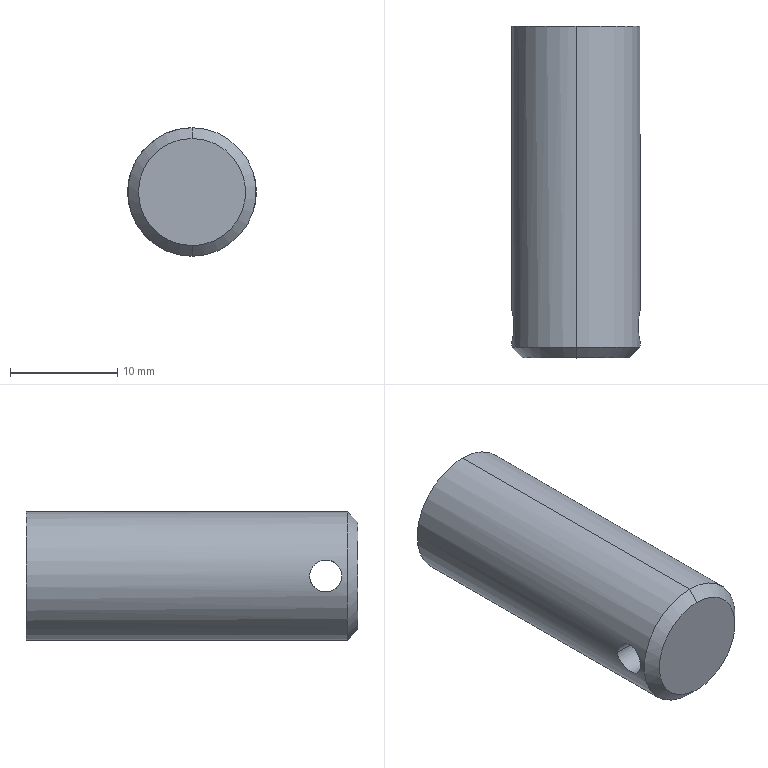Part | STEP file | Positioning_id990_x_t | 1 solid | 8 faces | box 12 x 31 x 12 mm | volume 3404 mm3 | cylinder 4 | cone 2 | plane 2 | commonest cylinder face diameters 3 x2 12 x2
STEP:
#1=CARTESIAN_POINT('',(0.,0.,0.));
#2=DIRECTION('',(0.,0.,1.));
#3=DIRECTION('',(1.,0.,0.));
#4=AXIS2_PLACEMENT_3D('',#1,#2,#3);
#5=CARTESIAN_POINT('',(-767.002,184.,187.532));
#6=VERTEX_POINT('',#5);
#7=CARTESIAN_POINT('',(-767.002,183.,188.532));
#8=VERTEX_POINT('',#7);
#9=CARTESIAN_POINT('',(-767.002,183.,188.532));
#10=DIRECTION('',(0.,-0.7071,0.7071));
#11=VECTOR('',#10,1.);
#12=LINE('',#9,#11);
#13=CARTESIAN_POINT('',(-767.002,184.,193.532));
#14=DIRECTION('',(0.,1.,0.));
#15=DIRECTION('',(0.,0.,-1.));
#16=AXIS2_PLACEMENT_3D('',#13,#14,#15);
#17=CONICAL_SURFACE('',#16,6.,0.7854);
#18=CARTESIAN_POINT('',(0.,-1.));
#19=DIRECTION('',(0.,-1.));
#20=VECTOR('',#19,1.);
#21=LINE('',#18,#20);
#22=(GEOMETRIC_REPRESENTATION_CONTEXT(2)PARAMETRIC_REPRESENTATION_CONTEXT()REPRESENTATION_CONTEXT('',''));
#23=DEFINITIONAL_REPRESENTATION('',(#21),#22);
#24=PCURVE('',#17,#23);
#25=CARTESIAN_POINT('',(-767.002,184.,193.532));
#26=DIRECTION('',(0.,1.,0.));
#27=DIRECTION('',(0.,0.,-1.));
#28=AXIS2_PLACEMENT_3D('',#25,#26,#27);
#29=CONICAL_SURFACE('',#28,6.,0.7854);
#30=CARTESIAN_POINT('',(6.283,-1.));
#31=DIRECTION('',(0.,-1.));
#32=VECTOR('',#31,1.);
#33=LINE('',#30,#32);
#34=(GEOMETRIC_REPRESENTATION_CONTEXT(2)PARAMETRIC_REPRESENTATION_CONTEXT()REPRESENTATION_CONTEXT('',''));
#35=DEFINITIONAL_REPRESENTATION('',(#33),#34);
#36=PCURVE('',#29,#35);
#37=SURFACE_CURVE('',#12,(#24,#36),.PCURVE_S1.);
#38=EDGE_CURVE('',#6,#8,#37,.T.);
#39=ORIENTED_EDGE('',*,*,#38,.T.);
#40=CARTESIAN_POINT('',(-767.002,183.,198.532));
#41=VERTEX_POINT('',#40);
#42=CARTESIAN_POINT('',(-767.002,183.,193.532));
#43=DIRECTION('',(0.,1.,0.));
#44=DIRECTION('',(0.,0.,1.));
#45=AXIS2_PLACEMENT_3D('',#42,#43,#44);
#46=CIRCLE('',#45,5.);
#47=CARTESIAN_POINT('',(-3.142,-1.));
#48=DIRECTION('',(1.,0.));
#49=VECTOR('',#48,1.);
#50=LINE('',#47,#49);
#51=(GEOMETRIC_REPRESENTATION_CONTEXT(2)PARAMETRIC_REPRESENTATION_CONTEXT()REPRESENTATION_CONTEXT('',''));
#52=DEFINITIONAL_REPRESENTATION('',(#50),#51);
#53=PCURVE('',#17,#52);
#54=CARTESIAN_POINT('',(-767.002,183.,193.532));
#55=DIRECTION('',(0.,-1.,0.));
#56=DIRECTION('',(0.,0.,-1.));
#57=AXIS2_PLACEMENT_3D('',#54,#55,#56);
#58=PLANE('',#57);
#59=CARTESIAN_POINT('',(-5.,0.));
#60=CARTESIAN_POINT('',(-5.,8.66));
#61=CARTESIAN_POINT('',(2.5,4.33));
#62=CARTESIAN_POINT('',(10.,0.));
#63=CARTESIAN_POINT('',(2.5,-4.33));
#64=CARTESIAN_POINT('',(-5.,-8.66));
#65=CARTESIAN_POINT('',(-5.,0.));
#66=(BOUNDED_CURVE()B_SPLINE_CURVE(2,(#59,#60,#61,#62,#63,#64,#65),.UNSPECIFIED.,.T.,.F.)B_SPLINE_CURVE_WITH_KNOTS((1,2,2,2,2,1),(-2.094,0.,2.094,4.189,6.283,8.378),.UNSPECIFIED.)CURVE()GEOMETRIC_REPRESENTATION_ITEM()RATIONAL_B_SPLINE_CURVE((1.,0.5,1.,0.5,1.,0.5,1.))REPRESENTATION_ITEM(''));
#67=(GEOMETRIC_REPRESENTATION_CONTEXT(2)PARAMETRIC_REPRESENTATION_CONTEXT()REPRESENTATION_CONTEXT('',''));
#68=DEFINITIONAL_REPRESENTATION('',(#66),#67);
#69=PCURVE('',#58,#68);
#70=SURFACE_CURVE('',#46,(#53,#69),.PCURVE_S1.);
#71=EDGE_CURVE('',#8,#41,#70,.T.);
#72=ORIENTED_EDGE('',*,*,#71,.T.);
#73=CARTESIAN_POINT('',(-767.002,184.,199.532));
#74=VERTEX_POINT('',#73);
#75=CARTESIAN_POINT('',(-767.002,183.,198.532));
#76=DIRECTION('',(0.,0.7071,0.7071));
#77=VECTOR('',#76,1.);
#78=LINE('',#75,#77);
#79=CARTESIAN_POINT('',(3.142,-1.));
#80=DIRECTION('',(0.,1.));
#81=VECTOR('',#80,1.);
#82=LINE('',#79,#81);
#83=(GEOMETRIC_REPRESENTATION_CONTEXT(2)PARAMETRIC_REPRESENTATION_CONTEXT()REPRESENTATION_CONTEXT('',''));
#84=DEFINITIONAL_REPRESENTATION('',(#82),#83);
#85=PCURVE('',#17,#84);
#86=CARTESIAN_POINT('',(3.142,-1.));
#87=DIRECTION('',(0.,1.));
#88=VECTOR('',#87,1.);
#89=LINE('',#86,#88);
#90=(GEOMETRIC_REPRESENTATION_CONTEXT(2)PARAMETRIC_REPRESENTATION_CONTEXT()REPRESENTATION_CONTEXT('',''));
#91=DEFINITIONAL_REPRESENTATION('',(#89),#90);
#92=PCURVE('',#29,#91);
#93=SURFACE_CURVE('',#78,(#85,#92),.PCURVE_S1.);
#94=EDGE_CURVE('',#41,#74,#93,.T.);
#95=ORIENTED_EDGE('',*,*,#94,.T.);
#96=CARTESIAN_POINT('',(-767.002,184.,193.532));
#97=DIRECTION('',(0.,-1.,0.));
#98=DIRECTION('',(0.,0.,1.));
#99=AXIS2_PLACEMENT_3D('',#96,#97,#98);
#100=CIRCLE('',#99,6.);
#101=CARTESIAN_POINT('',(3.142,0.));
#102=DIRECTION('',(-1.,0.));
#103=VECTOR('',#102,1.);
#104=LINE('',#101,#103);
#105=(GEOMETRIC_REPRESENTATION_CONTEXT(2)PARAMETRIC_REPRESENTATION_CONTEXT()REPRESENTATION_CONTEXT('',''));
#106=DEFINITIONAL_REPRESENTATION('',(#104),#105);
#107=PCURVE('',#17,#106);
#108=CARTESIAN_POINT('',(-767.002,214.,193.532));
#109=DIRECTION('',(0.,1.,0.));
#110=DIRECTION('',(0.,0.,-1.));
#111=AXIS2_PLACEMENT_3D('',#108,#109,#110);
#112=CYLINDRICAL_SURFACE('',#111,6.);
#113=CARTESIAN_POINT('',(3.142,-30.));
#114=DIRECTION('',(-1.,0.));
#115=VECTOR('',#114,1.);
#116=LINE('',#113,#115);
#117=(GEOMETRIC_REPRESENTATION_CONTEXT(2)PARAMETRIC_REPRESENTATION_CONTEXT()REPRESENTATION_CONTEXT('',''));
#118=DEFINITIONAL_REPRESENTATION('',(#116),#117);
#119=PCURVE('',#112,#118);
#120=SURFACE_CURVE('',#100,(#107,#119),.PCURVE_S1.);
#121=EDGE_CURVE('',#74,#6,#120,.T.);
#122=ORIENTED_EDGE('',*,*,#121,.T.);
#123=EDGE_LOOP('',(#39,#72,#95,#122));
#124=FACE_BOUND('',#123,.T.);
#125=ADVANCED_FACE('',(#124),#17,.T.);
#126=CARTESIAN_POINT('',(-773.002,184.5,193.532));
#127=VERTEX_POINT('',#126);
#128=CARTESIAN_POINT('',(-773.002,187.5,193.532));
#129=VERTEX_POINT('',#128);
#130=CARTESIAN_POINT('',(-773.002,184.5,193.532));
#131=CARTESIAN_POINT('',(-773.002,184.5,193.367));
#132=CARTESIAN_POINT('',(-772.995,184.528,193.2));
#133=CARTESIAN_POINT('',(-772.982,184.582,193.044));
#134=CARTESIAN_POINT('',(-772.969,184.635,192.888));
#135=CARTESIAN_POINT('',(-772.951,184.715,192.74));
#136=CARTESIAN_POINT('',(-772.931,184.816,192.611));
#137=CARTESIAN_POINT('',(-772.91,184.918,192.48));
#138=CARTESIAN_POINT('',(-772.888,185.044,192.364));
#139=CARTESIAN_POINT('',(-772.868,185.184,192.273));
#140=CARTESIAN_POINT('',(-772.849,185.326,192.181));
#141=CARTESIAN_POINT('',(-772.832,185.487,192.112));
#142=CARTESIAN_POINT('',(-772.822,185.652,192.073));
#143=CARTESIAN_POINT('',(-772.812,185.814,192.034));
#144=CARTESIAN_POINT('',(-772.809,185.986,192.023));
#145=CARTESIAN_POINT('',(-772.813,186.152,192.04));
#146=CARTESIAN_POINT('',(-772.818,186.314,192.056));
#147=CARTESIAN_POINT('',(-772.829,186.475,192.1));
#148=CARTESIAN_POINT('',(-772.845,186.623,192.167));
#149=CARTESIAN_POINT('',(-772.86,186.772,192.235));
#150=CARTESIAN_POINT('',(-772.881,186.911,192.329));
#151=CARTESIAN_POINT('',(-772.902,187.03,192.441));
#152=CARTESIAN_POINT('',(-772.923,187.152,192.557));
#153=CARTESIAN_POINT('',(-772.945,187.256,192.695));
#154=CARTESIAN_POINT('',(-772.962,187.333,192.844));
#155=CARTESIAN_POINT('',(-772.98,187.411,192.994));
#156=CARTESIAN_POINT('',(-772.993,187.463,193.161));
#157=CARTESIAN_POINT('',(-772.998,187.486,193.329));
#158=CARTESIAN_POINT('',(-773.001,187.495,193.396));
#159=CARTESIAN_POINT('',(-773.002,187.5,193.464));
#160=CARTESIAN_POINT('',(-773.002,187.5,193.532));
#161=B_SPLINE_CURVE_WITH_KNOTS('',3,(#130,#131,#132,#133,#134,#135,#136,#137,#138,#139,#140,#141,#142,#143,#144,#145,#146,#147,#148,#149,#150,#151,#152,#153,#154,#155,#156,#157,#158,#159,#160),.UNSPECIFIED.,.F.,.F.,(4,3,3,3,3,3,3,3,3,3,4),(0.,0.1052,0.2102,0.3173,0.4259,0.5324,0.6362,0.7411,0.849,0.9573,1.),.UNSPECIFIED.);
#162=CARTESIAN_POINT('',(-757.002,186.,193.532));
#163=DIRECTION('',(1.,0.,0.));
#164=DIRECTION('',(0.,-1.,0.));
#165=AXIS2_PLACEMENT_3D('',#162,#163,#164);
#166=CYLINDRICAL_SURFACE('',#165,1.5);
#167=CARTESIAN_POINT('',(0.,-16.));
#168=CARTESIAN_POINT('',(0.02377,-16.));
#169=CARTESIAN_POINT('',(0.07146,-15.999));
#170=CARTESIAN_POINT('',(0.1432,-15.996));
#171=CARTESIAN_POINT('',(0.215,-15.992));
#172=CARTESIAN_POINT('',(0.2866,-15.985));
#173=CARTESIAN_POINT('',(0.3577,-15.977));
#174=CARTESIAN_POINT('',(0.4291,-15.968));
#175=CARTESIAN_POINT('',(0.5006,-15.957));
#176=CARTESIAN_POINT('',(0.572,-15.945));
#177=CARTESIAN_POINT('',(0.6432,-15.932));
#178=CARTESIAN_POINT('',(0.714,-15.919));
#179=CARTESIAN_POINT('',(0.7852,-15.906));
#180=CARTESIAN_POINT('',(0.8564,-15.892));
#181=CARTESIAN_POINT('',(0.9277,-15.879));
#182=CARTESIAN_POINT('',(0.9986,-15.866));
#183=CARTESIAN_POINT('',(1.07,-15.854));
#184=CARTESIAN_POINT('',(1.141,-15.843));
#185=CARTESIAN_POINT('',(1.213,-15.833));
#186=CARTESIAN_POINT('',(1.284,-15.825));
#187=CARTESIAN_POINT('',(1.355,-15.818));
#188=CARTESIAN_POINT('',(1.427,-15.813));
#189=CARTESIAN_POINT('',(1.499,-15.81));
#190=CARTESIAN_POINT('',(1.57,-15.809));
#191=CARTESIAN_POINT('',(1.642,-15.81));
#192=CARTESIAN_POINT('',(1.713,-15.813));
#193=CARTESIAN_POINT('',(1.785,-15.818));
#194=CARTESIAN_POINT('',(1.857,-15.825));
#195=CARTESIAN_POINT('',(1.928,-15.833));
#196=CARTESIAN_POINT('',(1.999,-15.843));
#197=CARTESIAN_POINT('',(2.071,-15.854));
#198=CARTESIAN_POINT('',(2.142,-15.866));
#199=CARTESIAN_POINT('',(2.213,-15.879));
#200=CARTESIAN_POINT('',(2.285,-15.892));
#201=CARTESIAN_POINT('',(2.355,-15.905));
#202=CARTESIAN_POINT('',(2.426,-15.919));
#203=CARTESIAN_POINT('',(2.498,-15.932));
#204=CARTESIAN_POINT('',(2.569,-15.945));
#205=CARTESIAN_POINT('',(2.64,-15.957));
#206=CARTESIAN_POINT('',(2.711,-15.967));
#207=CARTESIAN_POINT('',(2.783,-15.977));
#208=CARTESIAN_POINT('',(2.854,-15.985));
#209=CARTESIAN_POINT('',(2.926,-15.992));
#210=CARTESIAN_POINT('',(2.997,-15.996));
#211=CARTESIAN_POINT('',(3.069,-15.999));
#212=CARTESIAN_POINT('',(3.118,-16.));
#213=CARTESIAN_POINT('',(3.142,-16.));
#214=B_SPLINE_CURVE_WITH_KNOTS('',3,(#167,#168,#169,#170,#171,#172,#173,#174,#175,#176,#177,#178,#179,#180,#181,#182,#183,#184,#185,#186,#187,#188,#189,#190,#191,#192,#193,#194,#195,#196,#197,#198,#199,#200,#201,#202,#203,#204,#205,#206,#207,#208,#209,#210,#211,#212,#213),.UNSPECIFIED.,.F.,.F.,(4,1,1,1,1,1,1,1,1,1,1,1,1,1,1,1,1,1,1,1,1,1,1,1,1,1,1,1,1,1,1,1,1,1,1,1,1,1,1,1,1,1,1,1,4),(0.,0.02273,0.04545,0.06818,0.09091,0.1136,0.1364,0.1591,0.1818,0.2045,0.2273,0.25,0.2727,0.2955,0.3182,0.3409,0.3636,0.3864,0.4091,0.4318,0.4545,0.4773,0.5,0.5227,0.5455,0.5682,0.5909,0.6136,0.6364,0.6591,0.6818,0.7045,0.7273,0.75,0.7727,0.7955,0.8182,0.8409,0.8636,0.8864,0.9091,0.9318,0.9545,0.9773,1.),.QUASI_UNIFORM_KNOTS.);
#215=(GEOMETRIC_REPRESENTATION_CONTEXT(2)PARAMETRIC_REPRESENTATION_CONTEXT()REPRESENTATION_CONTEXT('',''));
#216=DEFINITIONAL_REPRESENTATION('',(#214),#215);
#217=PCURVE('',#166,#216);
#218=CARTESIAN_POINT('',(1.571,-29.5));
#219=CARTESIAN_POINT('',(1.565,-29.5));
#220=CARTESIAN_POINT('',(1.553,-29.497));
#221=CARTESIAN_POINT('',(1.535,-29.486));
#222=CARTESIAN_POINT('',(1.517,-29.467));
#223=CARTESIAN_POINT('',(1.5,-29.44));
#224=CARTESIAN_POINT('',(1.483,-29.406));
#225=CARTESIAN_POINT('',(1.467,-29.365));
#226=CARTESIAN_POINT('',(1.45,-29.317));
#227=CARTESIAN_POINT('',(1.435,-29.262));
#228=CARTESIAN_POINT('',(1.42,-29.201));
#229=CARTESIAN_POINT('',(1.406,-29.135));
#230=CARTESIAN_POINT('',(1.393,-29.062));
#231=CARTESIAN_POINT('',(1.381,-28.983));
#232=CARTESIAN_POINT('',(1.369,-28.9));
#233=CARTESIAN_POINT('',(1.359,-28.813));
#234=CARTESIAN_POINT('',(1.35,-28.721));
#235=CARTESIAN_POINT('',(1.341,-28.625));
#236=CARTESIAN_POINT('',(1.334,-28.526));
#237=CARTESIAN_POINT('',(1.328,-28.425));
#238=CARTESIAN_POINT('',(1.324,-28.321));
#239=CARTESIAN_POINT('',(1.321,-28.216));
#240=CARTESIAN_POINT('',(1.319,-28.108));
#241=CARTESIAN_POINT('',(1.318,-28.001));
#242=CARTESIAN_POINT('',(1.319,-27.893));
#243=CARTESIAN_POINT('',(1.321,-27.787));
#244=CARTESIAN_POINT('',(1.324,-27.681));
#245=CARTESIAN_POINT('',(1.328,-27.577));
#246=CARTESIAN_POINT('',(1.334,-27.475));
#247=CARTESIAN_POINT('',(1.341,-27.376));
#248=CARTESIAN_POINT('',(1.349,-27.281));
#249=CARTESIAN_POINT('',(1.359,-27.188));
#250=CARTESIAN_POINT('',(1.369,-27.1));
#251=CARTESIAN_POINT('',(1.381,-27.017));
#252=CARTESIAN_POINT('',(1.393,-26.939));
#253=CARTESIAN_POINT('',(1.406,-26.867));
#254=CARTESIAN_POINT('',(1.42,-26.799));
#255=CARTESIAN_POINT('',(1.435,-26.738));
#256=CARTESIAN_POINT('',(1.45,-26.683));
#257=CARTESIAN_POINT('',(1.466,-26.636));
#258=CARTESIAN_POINT('',(1.483,-26.595));
#259=CARTESIAN_POINT('',(1.5,-26.56));
#260=CARTESIAN_POINT('',(1.517,-26.534));
#261=CARTESIAN_POINT('',(1.535,-26.514));
#262=CARTESIAN_POINT('',(1.553,-26.503));
#263=CARTESIAN_POINT('',(1.565,-26.5));
#264=CARTESIAN_POINT('',(1.571,-26.5));
#265=B_SPLINE_CURVE_WITH_KNOTS('',3,(#218,#219,#220,#221,#222,#223,#224,#225,#226,#227,#228,#229,#230,#231,#232,#233,#234,#235,#236,#237,#238,#239,#240,#241,#242,#243,#244,#245,#246,#247,#248,#249,#250,#251,#252,#253,#254,#255,#256,#257,#258,#259,#260,#261,#262,#263,#264),.UNSPECIFIED.,.F.,.F.,(4,1,1,1,1,1,1,1,1,1,1,1,1,1,1,1,1,1,1,1,1,1,1,1,1,1,1,1,1,1,1,1,1,1,1,1,1,1,1,1,1,1,1,1,4),(0.,0.02273,0.04545,0.06818,0.09091,0.1136,0.1364,0.1591,0.1818,0.2045,0.2273,0.25,0.2727,0.2955,0.3182,0.3409,0.3636,0.3864,0.4091,0.4318,0.4545,0.4773,0.5,0.5227,0.5455,0.5682,0.5909,0.6136,0.6364,0.6591,0.6818,0.7045,0.7273,0.75,0.7727,0.7955,0.8182,0.8409,0.8636,0.8864,0.9091,0.9318,0.9545,0.9773,1.),.QUASI_UNIFORM_KNOTS.);
#266=(GEOMETRIC_REPRESENTATION_CONTEXT(2)PARAMETRIC_REPRESENTATION_CONTEXT()REPRESENTATION_CONTEXT('',''));
#267=DEFINITIONAL_REPRESENTATION('',(#265),#266);
#268=PCURVE('',#112,#267);
#269=SURFACE_CURVE('',#161,(#217,#268),.PCURVE_S1.);
#270=EDGE_CURVE('',#127,#129,#269,.T.);
#271=ORIENTED_EDGE('',*,*,#270,.T.);
#272=CARTESIAN_POINT('',(-761.002,187.5,193.532));
#273=VERTEX_POINT('',#272);
#274=CARTESIAN_POINT('',(-761.002,187.5,193.532));
#275=DIRECTION('',(1.,0.,0.));
#276=VECTOR('',#275,1.);
#277=LINE('',#274,#276);
#278=CARTESIAN_POINT('',(3.142,-4.));
#279=DIRECTION('',(0.,1.));
#280=VECTOR('',#279,1.);
#281=LINE('',#278,#280);
#282=(GEOMETRIC_REPRESENTATION_CONTEXT(2)PARAMETRIC_REPRESENTATION_CONTEXT()REPRESENTATION_CONTEXT('',''));
#283=DEFINITIONAL_REPRESENTATION('',(#281),#282);
#284=PCURVE('',#166,#283);
#285=CARTESIAN_POINT('',(-757.002,186.,193.532));
#286=DIRECTION('',(1.,0.,0.));
#287=DIRECTION('',(0.,-1.,0.));
#288=AXIS2_PLACEMENT_3D('',#285,#286,#287);
#289=CYLINDRICAL_SURFACE('',#288,1.5);
#290=CARTESIAN_POINT('',(3.142,-4.));
#291=DIRECTION('',(0.,1.));
#292=VECTOR('',#291,1.);
#293=LINE('',#290,#292);
#294=(GEOMETRIC_REPRESENTATION_CONTEXT(2)PARAMETRIC_REPRESENTATION_CONTEXT()REPRESENTATION_CONTEXT('',''));
#295=DEFINITIONAL_REPRESENTATION('',(#293),#294);
#296=PCURVE('',#289,#295);
#297=SURFACE_CURVE('',#277,(#284,#296),.PCURVE_S1.);
#298=EDGE_CURVE('',#129,#273,#297,.T.);
#299=ORIENTED_EDGE('',*,*,#298,.T.);
#300=CARTESIAN_POINT('',(-761.002,184.5,193.532));
#301=VERTEX_POINT('',#300);
#302=CARTESIAN_POINT('',(-761.002,187.5,193.532));
#303=CARTESIAN_POINT('',(-761.002,187.5,193.367));
#304=CARTESIAN_POINT('',(-761.009,187.472,193.2));
#305=CARTESIAN_POINT('',(-761.022,187.418,193.044));
#306=CARTESIAN_POINT('',(-761.034,187.365,192.888));
#307=CARTESIAN_POINT('',(-761.053,187.285,192.74));
#308=CARTESIAN_POINT('',(-761.073,187.184,192.611));
#309=CARTESIAN_POINT('',(-761.093,187.082,192.48));
#310=CARTESIAN_POINT('',(-761.116,186.956,192.364));
#311=CARTESIAN_POINT('',(-761.135,186.816,192.273));
#312=CARTESIAN_POINT('',(-761.155,186.674,192.181));
#313=CARTESIAN_POINT('',(-761.172,186.513,192.112));
#314=CARTESIAN_POINT('',(-761.182,186.348,192.073));
#315=CARTESIAN_POINT('',(-761.192,186.186,192.034));
#316=CARTESIAN_POINT('',(-761.195,186.014,192.023));
#317=CARTESIAN_POINT('',(-761.19,185.848,192.04));
#318=CARTESIAN_POINT('',(-761.186,185.686,192.056));
#319=CARTESIAN_POINT('',(-761.175,185.525,192.1));
#320=CARTESIAN_POINT('',(-761.159,185.377,192.167));
#321=CARTESIAN_POINT('',(-761.143,185.228,192.235));
#322=CARTESIAN_POINT('',(-761.122,185.089,192.329));
#323=CARTESIAN_POINT('',(-761.102,184.97,192.441));
#324=CARTESIAN_POINT('',(-761.08,184.848,192.557));
#325=CARTESIAN_POINT('',(-761.059,184.744,192.695));
#326=CARTESIAN_POINT('',(-761.041,184.667,192.844));
#327=CARTESIAN_POINT('',(-761.024,184.589,192.994));
#328=CARTESIAN_POINT('',(-761.011,184.537,193.161));
#329=CARTESIAN_POINT('',(-761.005,184.514,193.329));
#330=CARTESIAN_POINT('',(-761.003,184.505,193.396));
#331=CARTESIAN_POINT('',(-761.002,184.5,193.464));
#332=CARTESIAN_POINT('',(-761.002,184.5,193.532));
#333=B_SPLINE_CURVE_WITH_KNOTS('',3,(#302,#303,#304,#305,#306,#307,#308,#309,#310,#311,#312,#313,#314,#315,#316,#317,#318,#319,#320,#321,#322,#323,#324,#325,#326,#327,#328,#329,#330,#331,#332),.UNSPECIFIED.,.F.,.F.,(4,3,3,3,3,3,3,3,3,3,4),(0.,0.1052,0.2102,0.3173,0.4259,0.5324,0.6362,0.7411,0.849,0.9573,1.),.UNSPECIFIED.);
#334=CARTESIAN_POINT('',(3.142,-4.));
#335=CARTESIAN_POINT('',(3.118,-4.));
#336=CARTESIAN_POINT('',(3.07,-4.001));
#337=CARTESIAN_POINT('',(2.998,-4.004));
#338=CARTESIAN_POINT('',(2.927,-4.008));
#339=CARTESIAN_POINT('',(2.855,-4.015));
#340=CARTESIAN_POINT('',(2.784,-4.023));
#341=CARTESIAN_POINT('',(2.712,-4.032));
#342=CARTESIAN_POINT('',(2.641,-4.043));
#343=CARTESIAN_POINT('',(2.57,-4.055));
#344=CARTESIAN_POINT('',(2.498,-4.068));
#345=CARTESIAN_POINT('',(2.428,-4.081));
#346=CARTESIAN_POINT('',(2.356,-4.094));
#347=CARTESIAN_POINT('',(2.285,-4.108));
#348=CARTESIAN_POINT('',(2.214,-4.121));
#349=CARTESIAN_POINT('',(2.143,-4.134));
#350=CARTESIAN_POINT('',(2.072,-4.146));
#351=CARTESIAN_POINT('',(2.001,-4.157));
#352=CARTESIAN_POINT('',(1.929,-4.167));
#353=CARTESIAN_POINT('',(1.858,-4.175));
#354=CARTESIAN_POINT('',(1.786,-4.182));
#355=CARTESIAN_POINT('',(1.715,-4.187));
#356=CARTESIAN_POINT('',(1.643,-4.19));
#357=CARTESIAN_POINT('',(1.571,-4.191));
#358=CARTESIAN_POINT('',(1.5,-4.19));
#359=CARTESIAN_POINT('',(1.428,-4.187));
#360=CARTESIAN_POINT('',(1.357,-4.182));
#361=CARTESIAN_POINT('',(1.285,-4.175));
#362=CARTESIAN_POINT('',(1.213,-4.167));
#363=CARTESIAN_POINT('',(1.142,-4.157));
#364=CARTESIAN_POINT('',(1.071,-4.146));
#365=CARTESIAN_POINT('',(0.9996,-4.134));
#366=CARTESIAN_POINT('',(0.9282,-4.121));
#367=CARTESIAN_POINT('',(0.857,-4.108));
#368=CARTESIAN_POINT('',(0.7863,-4.095));
#369=CARTESIAN_POINT('',(0.7152,-4.081));
#370=CARTESIAN_POINT('',(0.6439,-4.068));
#371=CARTESIAN_POINT('',(0.5726,-4.055));
#372=CARTESIAN_POINT('',(0.5014,-4.043));
#373=CARTESIAN_POINT('',(0.4305,-4.033));
#374=CARTESIAN_POINT('',(0.359,-4.023));
#375=CARTESIAN_POINT('',(0.2874,-4.015));
#376=CARTESIAN_POINT('',(0.2157,-4.008));
#377=CARTESIAN_POINT('',(0.1445,-4.004));
#378=CARTESIAN_POINT('',(0.07225,-4.001));
#379=CARTESIAN_POINT('',(0.02405,-4.));
#380=CARTESIAN_POINT('',(0.,-4.));
#381=B_SPLINE_CURVE_WITH_KNOTS('',3,(#334,#335,#336,#337,#338,#339,#340,#341,#342,#343,#344,#345,#346,#347,#348,#349,#350,#351,#352,#353,#354,#355,#356,#357,#358,#359,#360,#361,#362,#363,#364,#365,#366,#367,#368,#369,#370,#371,#372,#373,#374,#375,#376,#377,#378,#379,#380),.UNSPECIFIED.,.F.,.F.,(4,1,1,1,1,1,1,1,1,1,1,1,1,1,1,1,1,1,1,1,1,1,1,1,1,1,1,1,1,1,1,1,1,1,1,1,1,1,1,1,1,1,1,1,4),(0.,0.02273,0.04545,0.06818,0.09091,0.1136,0.1364,0.1591,0.1818,0.2045,0.2273,0.25,0.2727,0.2955,0.3182,0.3409,0.3636,0.3864,0.4091,0.4318,0.4545,0.4773,0.5,0.5227,0.5455,0.5682,0.5909,0.6136,0.6364,0.6591,0.6818,0.7045,0.7273,0.75,0.7727,0.7955,0.8182,0.8409,0.8636,0.8864,0.9091,0.9318,0.9545,0.9773,1.),.QUASI_UNIFORM_KNOTS.);
#382=(GEOMETRIC_REPRESENTATION_CONTEXT(2)PARAMETRIC_REPRESENTATION_CONTEXT()REPRESENTATION_CONTEXT('',''));
#383=DEFINITIONAL_REPRESENTATION('',(#381),#382);
#384=PCURVE('',#166,#383);
#385=CARTESIAN_POINT('',(-767.002,214.,193.532));
#386=DIRECTION('',(0.,1.,0.));
#387=DIRECTION('',(0.,0.,-1.));
#388=AXIS2_PLACEMENT_3D('',#385,#386,#387);
#389=CYLINDRICAL_SURFACE('',#388,6.);
#390=CARTESIAN_POINT('',(4.712,-26.5));
#391=CARTESIAN_POINT('',(4.718,-26.5));
#392=CARTESIAN_POINT('',(4.73,-26.503));
#393=CARTESIAN_POINT('',(4.748,-26.514));
#394=CARTESIAN_POINT('',(4.766,-26.533));
#395=CARTESIAN_POINT('',(4.783,-26.56));
#396=CARTESIAN_POINT('',(4.8,-26.594));
#397=CARTESIAN_POINT('',(4.817,-26.635));
#398=CARTESIAN_POINT('',(4.833,-26.683));
#399=CARTESIAN_POINT('',(4.848,-26.738));
#400=CARTESIAN_POINT('',(4.863,-26.799));
#401=CARTESIAN_POINT('',(4.877,-26.865));
#402=CARTESIAN_POINT('',(4.89,-26.938));
#403=CARTESIAN_POINT('',(4.903,-27.017));
#404=CARTESIAN_POINT('',(4.914,-27.1));
#405=CARTESIAN_POINT('',(4.924,-27.187));
#406=CARTESIAN_POINT('',(4.934,-27.279));
#407=CARTESIAN_POINT('',(4.942,-27.375));
#408=CARTESIAN_POINT('',(4.949,-27.474));
#409=CARTESIAN_POINT('',(4.955,-27.575));
#410=CARTESIAN_POINT('',(4.959,-27.679));
#411=CARTESIAN_POINT('',(4.963,-27.784));
#412=CARTESIAN_POINT('',(4.965,-27.892));
#413=CARTESIAN_POINT('',(4.965,-27.999));
#414=CARTESIAN_POINT('',(4.965,-28.107));
#415=CARTESIAN_POINT('',(4.963,-28.213));
#416=CARTESIAN_POINT('',(4.959,-28.319));
#417=CARTESIAN_POINT('',(4.955,-28.423));
#418=CARTESIAN_POINT('',(4.949,-28.525));
#419=CARTESIAN_POINT('',(4.942,-28.624));
#420=CARTESIAN_POINT('',(4.934,-28.719));
#421=CARTESIAN_POINT('',(4.924,-28.812));
#422=CARTESIAN_POINT('',(4.914,-28.9));
#423=CARTESIAN_POINT('',(4.903,-28.983));
#424=CARTESIAN_POINT('',(4.89,-29.061));
#425=CARTESIAN_POINT('',(4.877,-29.133));
#426=CARTESIAN_POINT('',(4.863,-29.201));
#427=CARTESIAN_POINT('',(4.848,-29.262));
#428=CARTESIAN_POINT('',(4.833,-29.317));
#429=CARTESIAN_POINT('',(4.817,-29.364));
#430=CARTESIAN_POINT('',(4.8,-29.405));
#431=CARTESIAN_POINT('',(4.783,-29.44));
#432=CARTESIAN_POINT('',(4.766,-29.466));
#433=CARTESIAN_POINT('',(4.748,-29.486));
#434=CARTESIAN_POINT('',(4.73,-29.497));
#435=CARTESIAN_POINT('',(4.718,-29.5));
#436=CARTESIAN_POINT('',(4.712,-29.5));
#437=B_SPLINE_CURVE_WITH_KNOTS('',3,(#390,#391,#392,#393,#394,#395,#396,#397,#398,#399,#400,#401,#402,#403,#404,#405,#406,#407,#408,#409,#410,#411,#412,#413,#414,#415,#416,#417,#418,#419,#420,#421,#422,#423,#424,#425,#426,#427,#428,#429,#430,#431,#432,#433,#434,#435,#436),.UNSPECIFIED.,.F.,.F.,(4,1,1,1,1,1,1,1,1,1,1,1,1,1,1,1,1,1,1,1,1,1,1,1,1,1,1,1,1,1,1,1,1,1,1,1,1,1,1,1,1,1,1,1,4),(0.,0.02273,0.04545,0.06818,0.09091,0.1136,0.1364,0.1591,0.1818,0.2045,0.2273,0.25,0.2727,0.2955,0.3182,0.3409,0.3636,0.3864,0.4091,0.4318,0.4545,0.4773,0.5,0.5227,0.5455,0.5682,0.5909,0.6136,0.6364,0.6591,0.6818,0.7045,0.7273,0.75,0.7727,0.7955,0.8182,0.8409,0.8636,0.8864,0.9091,0.9318,0.9545,0.9773,1.),.QUASI_UNIFORM_KNOTS.);
#438=(GEOMETRIC_REPRESENTATION_CONTEXT(2)PARAMETRIC_REPRESENTATION_CONTEXT()REPRESENTATION_CONTEXT('',''));
#439=DEFINITIONAL_REPRESENTATION('',(#437),#438);
#440=PCURVE('',#389,#439);
#441=SURFACE_CURVE('',#333,(#384,#440),.PCURVE_S1.);
#442=EDGE_CURVE('',#273,#301,#441,.T.);
#443=ORIENTED_EDGE('',*,*,#442,.T.);
#444=CARTESIAN_POINT('',(-761.002,184.5,193.532));
#445=DIRECTION('',(-1.,0.,0.));
#446=VECTOR('',#445,1.);
#447=LINE('',#444,#446);
#448=CARTESIAN_POINT('',(0.,-4.));
#449=DIRECTION('',(0.,-1.));
#450=VECTOR('',#449,1.);
#451=LINE('',#448,#450);
#452=(GEOMETRIC_REPRESENTATION_CONTEXT(2)PARAMETRIC_REPRESENTATION_CONTEXT()REPRESENTATION_CONTEXT('',''));
#453=DEFINITIONAL_REPRESENTATION('',(#451),#452);
#454=PCURVE('',#166,#453);
#455=CARTESIAN_POINT('',(6.283,-4.));
#456=DIRECTION('',(0.,-1.));
#457=VECTOR('',#456,1.);
#458=LINE('',#455,#457);
#459=(GEOMETRIC_REPRESENTATION_CONTEXT(2)PARAMETRIC_REPRESENTATION_CONTEXT()REPRESENTATION_CONTEXT('',''));
#460=DEFINITIONAL_REPRESENTATION('',(#458),#459);
#461=PCURVE('',#289,#460);
#462=SURFACE_CURVE('',#447,(#454,#461),.PCURVE_S1.);
#463=EDGE_CURVE('',#301,#127,#462,.T.);
#464=ORIENTED_EDGE('',*,*,#463,.T.);
#465=EDGE_LOOP('',(#271,#299,#443,#464));
#466=FACE_BOUND('',#465,.F.);
#467=ADVANCED_FACE('',(#466),#166,.F.);
#468=ORIENTED_EDGE('',*,*,#442,.T.);
#469=CARTESIAN_POINT('',(-761.002,184.5,193.532));
#470=CARTESIAN_POINT('',(-761.002,184.5,193.697));
#471=CARTESIAN_POINT('',(-761.009,184.528,193.864));
#472=CARTESIAN_POINT('',(-761.022,184.582,194.02));
#473=CARTESIAN_POINT('',(-761.034,184.635,194.175));
#474=CARTESIAN_POINT('',(-761.053,184.715,194.323));
#475=CARTESIAN_POINT('',(-761.073,184.816,194.453));
#476=CARTESIAN_POINT('',(-761.093,184.918,194.584));
#477=CARTESIAN_POINT('',(-761.116,185.044,194.7));
#478=CARTESIAN_POINT('',(-761.135,185.184,194.791));
#479=CARTESIAN_POINT('',(-761.155,185.326,194.883));
#480=CARTESIAN_POINT('',(-761.172,185.487,194.952));
#481=CARTESIAN_POINT('',(-761.182,185.652,194.991));
#482=CARTESIAN_POINT('',(-761.192,185.814,195.03));
#483=CARTESIAN_POINT('',(-761.195,185.986,195.041));
#484=CARTESIAN_POINT('',(-761.19,186.152,195.024));
#485=CARTESIAN_POINT('',(-761.186,186.314,195.008));
#486=CARTESIAN_POINT('',(-761.175,186.475,194.964));
#487=CARTESIAN_POINT('',(-761.159,186.623,194.896));
#488=CARTESIAN_POINT('',(-761.143,186.772,194.828));
#489=CARTESIAN_POINT('',(-761.122,186.911,194.735));
#490=CARTESIAN_POINT('',(-761.102,187.03,194.623));
#491=CARTESIAN_POINT('',(-761.08,187.152,194.507));
#492=CARTESIAN_POINT('',(-761.059,187.256,194.369));
#493=CARTESIAN_POINT('',(-761.041,187.333,194.219));
#494=CARTESIAN_POINT('',(-761.024,187.411,194.069));
#495=CARTESIAN_POINT('',(-761.011,187.463,193.903));
#496=CARTESIAN_POINT('',(-761.005,187.486,193.735));
#497=CARTESIAN_POINT('',(-761.003,187.495,193.668));
#498=CARTESIAN_POINT('',(-761.002,187.5,193.6));
#499=CARTESIAN_POINT('',(-761.002,187.5,193.532));
#500=B_SPLINE_CURVE_WITH_KNOTS('',3,(#469,#470,#471,#472,#473,#474,#475,#476,#477,#478,#479,#480,#481,#482,#483,#484,#485,#486,#487,#488,#489,#490,#491,#492,#493,#494,#495,#496,#497,#498,#499),.UNSPECIFIED.,.F.,.F.,(4,3,3,3,3,3,3,3,3,3,4),(0.,0.1052,0.2102,0.3173,0.4259,0.5324,0.6362,0.7411,0.849,0.9573,1.),.UNSPECIFIED.);
#501=CARTESIAN_POINT('',(4.712,-29.5));
#502=CARTESIAN_POINT('',(4.706,-29.5));
#503=CARTESIAN_POINT('',(4.695,-29.497));
#504=CARTESIAN_POINT('',(4.677,-29.486));
#505=CARTESIAN_POINT('',(4.659,-29.467));
#506=CARTESIAN_POINT('',(4.642,-29.44));
#507=CARTESIAN_POINT('',(4.625,-29.406));
#508=CARTESIAN_POINT('',(4.608,-29.365));
#509=CARTESIAN_POINT('',(4.592,-29.317));
#510=CARTESIAN_POINT('',(4.577,-29.262));
#511=CARTESIAN_POINT('',(4.562,-29.201));
#512=CARTESIAN_POINT('',(4.548,-29.135));
#513=CARTESIAN_POINT('',(4.535,-29.062));
#514=CARTESIAN_POINT('',(4.522,-28.983));
#515=CARTESIAN_POINT('',(4.511,-28.9));
#516=CARTESIAN_POINT('',(4.5,-28.813));
#517=CARTESIAN_POINT('',(4.491,-28.721));
#518=CARTESIAN_POINT('',(4.483,-28.625));
#519=CARTESIAN_POINT('',(4.476,-28.526));
#520=CARTESIAN_POINT('',(4.47,-28.425));
#521=CARTESIAN_POINT('',(4.465,-28.321));
#522=CARTESIAN_POINT('',(4.462,-28.216));
#523=CARTESIAN_POINT('',(4.46,-28.108));
#524=CARTESIAN_POINT('',(4.46,-28.001));
#525=CARTESIAN_POINT('',(4.46,-27.893));
#526=CARTESIAN_POINT('',(4.462,-27.787));
#527=CARTESIAN_POINT('',(4.465,-27.681));
#528=CARTESIAN_POINT('',(4.47,-27.577));
#529=CARTESIAN_POINT('',(4.476,-27.475));
#530=CARTESIAN_POINT('',(4.483,-27.376));
#531=CARTESIAN_POINT('',(4.491,-27.281));
#532=CARTESIAN_POINT('',(4.5,-27.188));
#533=CARTESIAN_POINT('',(4.511,-27.1));
#534=CARTESIAN_POINT('',(4.522,-27.017));
#535=CARTESIAN_POINT('',(4.534,-26.939));
#536=CARTESIAN_POINT('',(4.548,-26.867));
#537=CARTESIAN_POINT('',(4.562,-26.799));
#538=CARTESIAN_POINT('',(4.576,-26.738));
#539=CARTESIAN_POINT('',(4.592,-26.683));
#540=CARTESIAN_POINT('',(4.608,-26.636));
#541=CARTESIAN_POINT('',(4.624,-26.595));
#542=CARTESIAN_POINT('',(4.641,-26.56));
#543=CARTESIAN_POINT('',(4.659,-26.534));
#544=CARTESIAN_POINT('',(4.676,-26.514));
#545=CARTESIAN_POINT('',(4.694,-26.503));
#546=CARTESIAN_POINT('',(4.706,-26.5));
#547=CARTESIAN_POINT('',(4.712,-26.5));
#548=B_SPLINE_CURVE_WITH_KNOTS('',3,(#501,#502,#503,#504,#505,#506,#507,#508,#509,#510,#511,#512,#513,#514,#515,#516,#517,#518,#519,#520,#521,#522,#523,#524,#525,#526,#527,#528,#529,#530,#531,#532,#533,#534,#535,#536,#537,#538,#539,#540,#541,#542,#543,#544,#545,#546,#547),.UNSPECIFIED.,.F.,.F.,(4,1,1,1,1,1,1,1,1,1,1,1,1,1,1,1,1,1,1,1,1,1,1,1,1,1,1,1,1,1,1,1,1,1,1,1,1,1,1,1,1,1,1,1,4),(0.,0.02273,0.04545,0.06818,0.09091,0.1136,0.1364,0.1591,0.1818,0.2045,0.2273,0.25,0.2727,0.2955,0.3182,0.3409,0.3636,0.3864,0.4091,0.4318,0.4545,0.4773,0.5,0.5227,0.5455,0.5682,0.5909,0.6136,0.6364,0.6591,0.6818,0.7045,0.7273,0.75,0.7727,0.7955,0.8182,0.8409,0.8636,0.8864,0.9091,0.9318,0.9545,0.9773,1.),.QUASI_UNIFORM_KNOTS.);
#549=(GEOMETRIC_REPRESENTATION_CONTEXT(2)PARAMETRIC_REPRESENTATION_CONTEXT()REPRESENTATION_CONTEXT('',''));
#550=DEFINITIONAL_REPRESENTATION('',(#548),#549);
#551=PCURVE('',#389,#550);
#552=CARTESIAN_POINT('',(6.283,-4.));
#553=CARTESIAN_POINT('',(6.259,-4.));
#554=CARTESIAN_POINT('',(6.212,-4.001));
#555=CARTESIAN_POINT('',(6.14,-4.004));
#556=CARTESIAN_POINT('',(6.068,-4.008));
#557=CARTESIAN_POINT('',(5.997,-4.015));
#558=CARTESIAN_POINT('',(5.925,-4.023));
#559=CARTESIAN_POINT('',(5.854,-4.032));
#560=CARTESIAN_POINT('',(5.783,-4.043));
#561=CARTESIAN_POINT('',(5.711,-4.055));
#562=CARTESIAN_POINT('',(5.64,-4.068));
#563=CARTESIAN_POINT('',(5.569,-4.081));
#564=CARTESIAN_POINT('',(5.498,-4.094));
#565=CARTESIAN_POINT('',(5.427,-4.108));
#566=CARTESIAN_POINT('',(5.355,-4.121));
#567=CARTESIAN_POINT('',(5.285,-4.134));
#568=CARTESIAN_POINT('',(5.214,-4.146));
#569=CARTESIAN_POINT('',(5.142,-4.157));
#570=CARTESIAN_POINT('',(5.071,-4.167));
#571=CARTESIAN_POINT('',(4.999,-4.175));
#572=CARTESIAN_POINT('',(4.928,-4.182));
#573=CARTESIAN_POINT('',(4.856,-4.187));
#574=CARTESIAN_POINT('',(4.785,-4.19));
#575=CARTESIAN_POINT('',(4.713,-4.191));
#576=CARTESIAN_POINT('',(4.641,-4.19));
#577=CARTESIAN_POINT('',(4.57,-4.187));
#578=CARTESIAN_POINT('',(4.498,-4.182));
#579=CARTESIAN_POINT('',(4.427,-4.175));
#580=CARTESIAN_POINT('',(4.355,-4.167));
#581=CARTESIAN_POINT('',(4.284,-4.157));
#582=CARTESIAN_POINT('',(4.213,-4.146));
#583=CARTESIAN_POINT('',(4.141,-4.134));
#584=CARTESIAN_POINT('',(4.07,-4.121));
#585=CARTESIAN_POINT('',(3.999,-4.108));
#586=CARTESIAN_POINT('',(3.928,-4.095));
#587=CARTESIAN_POINT('',(3.857,-4.081));
#588=CARTESIAN_POINT('',(3.785,-4.068));
#589=CARTESIAN_POINT('',(3.714,-4.055));
#590=CARTESIAN_POINT('',(3.643,-4.043));
#591=CARTESIAN_POINT('',(3.572,-4.033));
#592=CARTESIAN_POINT('',(3.501,-4.023));
#593=CARTESIAN_POINT('',(3.429,-4.015));
#594=CARTESIAN_POINT('',(3.357,-4.008));
#595=CARTESIAN_POINT('',(3.286,-4.004));
#596=CARTESIAN_POINT('',(3.214,-4.001));
#597=CARTESIAN_POINT('',(3.166,-4.));
#598=CARTESIAN_POINT('',(3.142,-4.));
#599=B_SPLINE_CURVE_WITH_KNOTS('',3,(#552,#553,#554,#555,#556,#557,#558,#559,#560,#561,#562,#563,#564,#565,#566,#567,#568,#569,#570,#571,#572,#573,#574,#575,#576,#577,#578,#579,#580,#581,#582,#583,#584,#585,#586,#587,#588,#589,#590,#591,#592,#593,#594,#595,#596,#597,#598),.UNSPECIFIED.,.F.,.F.,(4,1,1,1,1,1,1,1,1,1,1,1,1,1,1,1,1,1,1,1,1,1,1,1,1,1,1,1,1,1,1,1,1,1,1,1,1,1,1,1,1,1,1,1,4),(0.,0.02273,0.04545,0.06818,0.09091,0.1136,0.1364,0.1591,0.1818,0.2045,0.2273,0.25,0.2727,0.2955,0.3182,0.3409,0.3636,0.3864,0.4091,0.4318,0.4545,0.4773,0.5,0.5227,0.5455,0.5682,0.5909,0.6136,0.6364,0.6591,0.6818,0.7045,0.7273,0.75,0.7727,0.7955,0.8182,0.8409,0.8636,0.8864,0.9091,0.9318,0.9545,0.9773,1.),.QUASI_UNIFORM_KNOTS.);
#600=(GEOMETRIC_REPRESENTATION_CONTEXT(2)PARAMETRIC_REPRESENTATION_CONTEXT()REPRESENTATION_CONTEXT('',''));
#601=DEFINITIONAL_REPRESENTATION('',(#599),#600);
#602=PCURVE('',#289,#601);
#603=SURFACE_CURVE('',#500,(#551,#602),.PCURVE_S1.);
#604=EDGE_CURVE('',#301,#273,#603,.T.);
#605=ORIENTED_EDGE('',*,*,#604,.T.);
#606=EDGE_LOOP('',(#468,#605));
#607=FACE_BOUND('',#606,.T.);
#608=CARTESIAN_POINT('',(-767.002,214.,187.532));
#609=VERTEX_POINT('',#608);
#610=CARTESIAN_POINT('',(-767.002,214.,187.532));
#611=DIRECTION('',(0.,1.,0.));
#612=VECTOR('',#611,1.);
#613=LINE('',#610,#612);
#614=CARTESIAN_POINT('',(6.283,0.));
#615=DIRECTION('',(0.,1.));
#616=VECTOR('',#615,1.);
#617=LINE('',#614,#616);
#618=(GEOMETRIC_REPRESENTATION_CONTEXT(2)PARAMETRIC_REPRESENTATION_CONTEXT()REPRESENTATION_CONTEXT('',''));
#619=DEFINITIONAL_REPRESENTATION('',(#617),#618);
#620=PCURVE('',#389,#619);
#621=CARTESIAN_POINT('',(0.,0.));
#622=DIRECTION('',(0.,1.));
#623=VECTOR('',#622,1.);
#624=LINE('',#621,#623);
#625=(GEOMETRIC_REPRESENTATION_CONTEXT(2)PARAMETRIC_REPRESENTATION_CONTEXT()REPRESENTATION_CONTEXT('',''));
#626=DEFINITIONAL_REPRESENTATION('',(#624),#625);
#627=PCURVE('',#112,#626);
#628=SURFACE_CURVE('',#613,(#620,#627),.PCURVE_S1.);
#629=EDGE_CURVE('',#6,#609,#628,.T.);
#630=ORIENTED_EDGE('',*,*,#629,.T.);
#631=CARTESIAN_POINT('',(-767.002,214.,199.532));
#632=VERTEX_POINT('',#631);
#633=CARTESIAN_POINT('',(-767.002,214.,193.532));
#634=DIRECTION('',(0.,1.,0.));
#635=DIRECTION('',(0.,0.,1.));
#636=AXIS2_PLACEMENT_3D('',#633,#634,#635);
#637=CIRCLE('',#636,6.);
#638=CARTESIAN_POINT('',(3.142,0.));
#639=DIRECTION('',(1.,0.));
#640=VECTOR('',#639,1.);
#641=LINE('',#638,#640);
#642=(GEOMETRIC_REPRESENTATION_CONTEXT(2)PARAMETRIC_REPRESENTATION_CONTEXT()REPRESENTATION_CONTEXT('',''));
#643=DEFINITIONAL_REPRESENTATION('',(#641),#642);
#644=PCURVE('',#389,#643);
#645=CARTESIAN_POINT('',(-767.002,214.,193.532));
#646=DIRECTION('',(0.,1.,0.));
#647=DIRECTION('',(0.,0.,1.));
#648=AXIS2_PLACEMENT_3D('',#645,#646,#647);
#649=PLANE('',#648);
#650=CARTESIAN_POINT('',(0.,0.));
#651=DIRECTION('',(1.,0.));
#652=AXIS2_PLACEMENT_2D('',#650,#651);
#653=CIRCLE('',#652,6.);
#654=(GEOMETRIC_REPRESENTATION_CONTEXT(2)PARAMETRIC_REPRESENTATION_CONTEXT()REPRESENTATION_CONTEXT('',''));
#655=DEFINITIONAL_REPRESENTATION('',(#653),#654);
#656=PCURVE('',#649,#655);
#657=SURFACE_CURVE('',#637,(#644,#656),.PCURVE_S1.);
#658=EDGE_CURVE('',#632,#609,#657,.T.);
#659=ORIENTED_EDGE('',*,*,#658,.F.);
#660=CARTESIAN_POINT('',(-767.002,214.,199.532));
#661=DIRECTION('',(0.,-1.,0.));
#662=VECTOR('',#661,1.);
#663=LINE('',#660,#662);
#664=CARTESIAN_POINT('',(3.142,0.));
#665=DIRECTION('',(0.,-1.));
#666=VECTOR('',#665,1.);
#667=LINE('',#664,#666);
#668=(GEOMETRIC_REPRESENTATION_CONTEXT(2)PARAMETRIC_REPRESENTATION_CONTEXT()REPRESENTATION_CONTEXT('',''));
#669=DEFINITIONAL_REPRESENTATION('',(#667),#668);
#670=PCURVE('',#389,#669);
#671=CARTESIAN_POINT('',(3.142,0.));
#672=DIRECTION('',(0.,-1.));
#673=VECTOR('',#672,1.);
#674=LINE('',#671,#673);
#675=(GEOMETRIC_REPRESENTATION_CONTEXT(2)PARAMETRIC_REPRESENTATION_CONTEXT()REPRESENTATION_CONTEXT('',''));
#676=DEFINITIONAL_REPRESENTATION('',(#674),#675);
#677=PCURVE('',#112,#676);
#678=SURFACE_CURVE('',#663,(#670,#677),.PCURVE_S1.);
#679=EDGE_CURVE('',#632,#74,#678,.T.);
#680=ORIENTED_EDGE('',*,*,#679,.T.);
#681=CARTESIAN_POINT('',(-767.002,184.,193.532));
#682=DIRECTION('',(0.,-1.,0.));
#683=DIRECTION('',(0.,0.,-1.));
#684=AXIS2_PLACEMENT_3D('',#681,#682,#683);
#685=CIRCLE('',#684,6.);
#686=CARTESIAN_POINT('',(6.283,-30.));
#687=DIRECTION('',(-1.,0.));
#688=VECTOR('',#687,1.);
#689=LINE('',#686,#688);
#690=(GEOMETRIC_REPRESENTATION_CONTEXT(2)PARAMETRIC_REPRESENTATION_CONTEXT()REPRESENTATION_CONTEXT('',''));
#691=DEFINITIONAL_REPRESENTATION('',(#689),#690);
#692=PCURVE('',#389,#691);
#693=CARTESIAN_POINT('',(6.283,0.));
#694=DIRECTION('',(-1.,0.));
#695=VECTOR('',#694,1.);
#696=LINE('',#693,#695);
#697=(GEOMETRIC_REPRESENTATION_CONTEXT(2)PARAMETRIC_REPRESENTATION_CONTEXT()REPRESENTATION_CONTEXT('',''));
#698=DEFINITIONAL_REPRESENTATION('',(#696),#697);
#699=PCURVE('',#29,#698);
#700=SURFACE_CURVE('',#685,(#692,#699),.PCURVE_S1.);
#701=EDGE_CURVE('',#6,#74,#700,.T.);
#702=ORIENTED_EDGE('',*,*,#701,.F.);
#703=EDGE_LOOP('',(#630,#659,#680,#702));
#704=FACE_BOUND('',#703,.T.);
#705=ADVANCED_FACE('',(#607,#704),#389,.T.);
#706=ORIENTED_EDGE('',*,*,#658,.T.);
#707=CARTESIAN_POINT('',(-767.002,214.,187.532));
#708=CARTESIAN_POINT('',(-773.002,214.,187.532));
#709=CARTESIAN_POINT('',(-776.002,214.,193.532));
#710=CARTESIAN_POINT('',(-773.002,214.,199.532));
#711=CARTESIAN_POINT('',(-767.002,214.,199.532));
#712=(BOUNDED_CURVE()B_SPLINE_CURVE(4,(#707,#708,#709,#710,#711),.UNSPECIFIED.,.F.,.F.)B_SPLINE_CURVE_WITH_KNOTS((5,5),(0.,1.),.PIECEWISE_BEZIER_KNOTS.)CURVE()GEOMETRIC_REPRESENTATION_ITEM()RATIONAL_B_SPLINE_CURVE((1.,0.7071,0.6667,0.7071,1.))REPRESENTATION_ITEM(''));
#713=CARTESIAN_POINT('',(-6.,0.));
#714=CARTESIAN_POINT('',(-6.,-6.));
#715=CARTESIAN_POINT('',(0.,-9.));
#716=CARTESIAN_POINT('',(6.,-6.));
#717=CARTESIAN_POINT('',(6.,0.));
#718=(BOUNDED_CURVE()B_SPLINE_CURVE(4,(#713,#714,#715,#716,#717),.UNSPECIFIED.,.F.,.F.)B_SPLINE_CURVE_WITH_KNOTS((5,5),(0.,1.),.PIECEWISE_BEZIER_KNOTS.)CURVE()GEOMETRIC_REPRESENTATION_ITEM()RATIONAL_B_SPLINE_CURVE((1.,0.7071,0.6667,0.7071,1.))REPRESENTATION_ITEM(''));
#719=(GEOMETRIC_REPRESENTATION_CONTEXT(2)PARAMETRIC_REPRESENTATION_CONTEXT()REPRESENTATION_CONTEXT('',''));
#720=DEFINITIONAL_REPRESENTATION('',(#718),#719);
#721=PCURVE('',#649,#720);
#722=CARTESIAN_POINT('',(0.,0.));
#723=CARTESIAN_POINT('',(0.04285,0.));
#724=CARTESIAN_POINT('',(0.1297,0.));
#725=CARTESIAN_POINT('',(0.2633,0.));
#726=CARTESIAN_POINT('',(0.3999,0.));
#727=CARTESIAN_POINT('',(0.5394,0.));
#728=CARTESIAN_POINT('',(0.6816,0.));
#729=CARTESIAN_POINT('',(0.8261,0.));
#730=CARTESIAN_POINT('',(0.9725,0.));
#731=CARTESIAN_POINT('',(1.121,0.));
#732=CARTESIAN_POINT('',(1.27,0.));
#733=CARTESIAN_POINT('',(1.42,0.));
#734=CARTESIAN_POINT('',(1.571,0.));
#735=CARTESIAN_POINT('',(1.721,0.));
#736=CARTESIAN_POINT('',(1.872,0.));
#737=CARTESIAN_POINT('',(2.021,0.));
#738=CARTESIAN_POINT('',(2.169,0.));
#739=CARTESIAN_POINT('',(2.316,0.));
#740=CARTESIAN_POINT('',(2.46,0.));
#741=CARTESIAN_POINT('',(2.602,0.));
#742=CARTESIAN_POINT('',(2.742,0.));
#743=CARTESIAN_POINT('',(2.878,0.));
#744=CARTESIAN_POINT('',(3.012,0.));
#745=CARTESIAN_POINT('',(3.099,0.));
#746=CARTESIAN_POINT('',(3.142,0.));
#747=B_SPLINE_CURVE_WITH_KNOTS('',3,(#722,#723,#724,#725,#726,#727,#728,#729,#730,#731,#732,#733,#734,#735,#736,#737,#738,#739,#740,#741,#742,#743,#744,#745,#746),.UNSPECIFIED.,.F.,.F.,(4,1,1,1,1,1,1,1,1,1,1,1,1,1,1,1,1,1,1,1,1,1,4),(0.,0.04545,0.09091,0.1364,0.1818,0.2273,0.2727,0.3182,0.3636,0.4091,0.4545,0.5,0.5455,0.5909,0.6364,0.6818,0.7273,0.7727,0.8182,0.8636,0.9091,0.9545,1.),.QUASI_UNIFORM_KNOTS.);
#748=(GEOMETRIC_REPRESENTATION_CONTEXT(2)PARAMETRIC_REPRESENTATION_CONTEXT()REPRESENTATION_CONTEXT('',''));
#749=DEFINITIONAL_REPRESENTATION('',(#747),#748);
#750=PCURVE('',#112,#749);
#751=SURFACE_CURVE('',#712,(#721,#750),.PCURVE_S1.);
#752=EDGE_CURVE('',#609,#632,#751,.T.);
#753=ORIENTED_EDGE('',*,*,#752,.T.);
#754=EDGE_LOOP('',(#706,#753));
#755=FACE_BOUND('',#754,.T.);
#756=ADVANCED_FACE('',(#755),#649,.T.);
#757=CARTESIAN_POINT('',(-767.002,183.,198.532));
#758=CARTESIAN_POINT('',(-762.002,183.,198.532));
#759=CARTESIAN_POINT('',(-759.502,183.,193.532));
#760=CARTESIAN_POINT('',(-762.002,183.,188.532));
#761=CARTESIAN_POINT('',(-767.002,183.,188.532));
#762=(BOUNDED_CURVE()B_SPLINE_CURVE(4,(#757,#758,#759,#760,#761),.UNSPECIFIED.,.F.,.F.)B_SPLINE_CURVE_WITH_KNOTS((5,5),(0.,1.),.PIECEWISE_BEZIER_KNOTS.)CURVE()GEOMETRIC_REPRESENTATION_ITEM()RATIONAL_B_SPLINE_CURVE((1.,0.7071,0.6667,0.7071,1.))REPRESENTATION_ITEM(''));
#763=CARTESIAN_POINT('',(-5.,0.));
#764=CARTESIAN_POINT('',(-5.,5.));
#765=CARTESIAN_POINT('',(0.,7.5));
#766=CARTESIAN_POINT('',(5.,5.));
#767=CARTESIAN_POINT('',(5.,0.));
#768=(BOUNDED_CURVE()B_SPLINE_CURVE(4,(#763,#764,#765,#766,#767),.UNSPECIFIED.,.F.,.F.)B_SPLINE_CURVE_WITH_KNOTS((5,5),(0.,1.),.PIECEWISE_BEZIER_KNOTS.)CURVE()GEOMETRIC_REPRESENTATION_ITEM()RATIONAL_B_SPLINE_CURVE((1.,0.7071,0.6667,0.7071,1.))REPRESENTATION_ITEM(''));
#769=(GEOMETRIC_REPRESENTATION_CONTEXT(2)PARAMETRIC_REPRESENTATION_CONTEXT()REPRESENTATION_CONTEXT('',''));
#770=DEFINITIONAL_REPRESENTATION('',(#768),#769);
#771=PCURVE('',#58,#770);
#772=CARTESIAN_POINT('',(3.142,-1.));
#773=CARTESIAN_POINT('',(3.184,-1.));
#774=CARTESIAN_POINT('',(3.271,-1.));
#775=CARTESIAN_POINT('',(3.405,-1.));
#776=CARTESIAN_POINT('',(3.542,-1.));
#777=CARTESIAN_POINT('',(3.681,-1.));
#778=CARTESIAN_POINT('',(3.823,-1.));
#779=CARTESIAN_POINT('',(3.968,-1.));
#780=CARTESIAN_POINT('',(4.114,-1.));
#781=CARTESIAN_POINT('',(4.262,-1.));
#782=CARTESIAN_POINT('',(4.412,-1.));
#783=CARTESIAN_POINT('',(4.562,-1.));
#784=CARTESIAN_POINT('',(4.712,-1.));
#785=CARTESIAN_POINT('',(4.863,-1.));
#786=CARTESIAN_POINT('',(5.013,-1.));
#787=CARTESIAN_POINT('',(5.163,-1.));
#788=CARTESIAN_POINT('',(5.311,-1.));
#789=CARTESIAN_POINT('',(5.457,-1.));
#790=CARTESIAN_POINT('',(5.602,-1.));
#791=CARTESIAN_POINT('',(5.744,-1.));
#792=CARTESIAN_POINT('',(5.883,-1.));
#793=CARTESIAN_POINT('',(6.02,-1.));
#794=CARTESIAN_POINT('',(6.153,-1.));
#795=CARTESIAN_POINT('',(6.24,-1.));
#796=CARTESIAN_POINT('',(6.283,-1.));
#797=B_SPLINE_CURVE_WITH_KNOTS('',3,(#772,#773,#774,#775,#776,#777,#778,#779,#780,#781,#782,#783,#784,#785,#786,#787,#788,#789,#790,#791,#792,#793,#794,#795,#796),.UNSPECIFIED.,.F.,.F.,(4,1,1,1,1,1,1,1,1,1,1,1,1,1,1,1,1,1,1,1,1,1,4),(0.,0.04545,0.09091,0.1364,0.1818,0.2273,0.2727,0.3182,0.3636,0.4091,0.4545,0.5,0.5455,0.5909,0.6364,0.6818,0.7273,0.7727,0.8182,0.8636,0.9091,0.9545,1.),.QUASI_UNIFORM_KNOTS.);
#798=(GEOMETRIC_REPRESENTATION_CONTEXT(2)PARAMETRIC_REPRESENTATION_CONTEXT()REPRESENTATION_CONTEXT('',''));
#799=DEFINITIONAL_REPRESENTATION('',(#797),#798);
#800=PCURVE('',#29,#799);
#801=SURFACE_CURVE('',#762,(#771,#800),.PCURVE_S1.);
#802=EDGE_CURVE('',#41,#8,#801,.T.);
#803=ORIENTED_EDGE('',*,*,#802,.F.);
#804=ORIENTED_EDGE('',*,*,#71,.F.);
#805=EDGE_LOOP('',(#803,#804));
#806=FACE_BOUND('',#805,.T.);
#807=ADVANCED_FACE('',(#806),#58,.T.);
#808=CARTESIAN_POINT('',(-773.002,187.5,193.532));
#809=CARTESIAN_POINT('',(-773.002,187.5,193.697));
#810=CARTESIAN_POINT('',(-772.995,187.472,193.864));
#811=CARTESIAN_POINT('',(-772.982,187.418,194.02));
#812=CARTESIAN_POINT('',(-772.969,187.365,194.175));
#813=CARTESIAN_POINT('',(-772.951,187.285,194.323));
#814=CARTESIAN_POINT('',(-772.931,187.184,194.453));
#815=CARTESIAN_POINT('',(-772.91,187.082,194.584));
#816=CARTESIAN_POINT('',(-772.888,186.956,194.7));
#817=CARTESIAN_POINT('',(-772.868,186.816,194.791));
#818=CARTESIAN_POINT('',(-772.849,186.674,194.883));
#819=CARTESIAN_POINT('',(-772.832,186.513,194.952));
#820=CARTESIAN_POINT('',(-772.822,186.348,194.991));
#821=CARTESIAN_POINT('',(-772.812,186.186,195.03));
#822=CARTESIAN_POINT('',(-772.809,186.014,195.041));
#823=CARTESIAN_POINT('',(-772.813,185.848,195.024));
#824=CARTESIAN_POINT('',(-772.818,185.686,195.008));
#825=CARTESIAN_POINT('',(-772.829,185.525,194.964));
#826=CARTESIAN_POINT('',(-772.845,185.377,194.896));
#827=CARTESIAN_POINT('',(-772.86,185.228,194.828));
#828=CARTESIAN_POINT('',(-772.881,185.089,194.735));
#829=CARTESIAN_POINT('',(-772.902,184.97,194.623));
#830=CARTESIAN_POINT('',(-772.923,184.848,194.507));
#831=CARTESIAN_POINT('',(-772.945,184.744,194.369));
#832=CARTESIAN_POINT('',(-772.962,184.667,194.219));
#833=CARTESIAN_POINT('',(-772.98,184.589,194.069));
#834=CARTESIAN_POINT('',(-772.993,184.537,193.903));
#835=CARTESIAN_POINT('',(-772.998,184.514,193.735));
#836=CARTESIAN_POINT('',(-773.001,184.505,193.668));
#837=CARTESIAN_POINT('',(-773.002,184.5,193.6));
#838=CARTESIAN_POINT('',(-773.002,184.5,193.532));
#839=B_SPLINE_CURVE_WITH_KNOTS('',3,(#808,#809,#810,#811,#812,#813,#814,#815,#816,#817,#818,#819,#820,#821,#822,#823,#824,#825,#826,#827,#828,#829,#830,#831,#832,#833,#834,#835,#836,#837,#838),.UNSPECIFIED.,.F.,.F.,(4,3,3,3,3,3,3,3,3,3,4),(0.,0.1052,0.2102,0.3173,0.4259,0.5324,0.6362,0.7411,0.849,0.9573,1.),.UNSPECIFIED.);
#840=CARTESIAN_POINT('',(1.571,-26.5));
#841=CARTESIAN_POINT('',(1.577,-26.5));
#842=CARTESIAN_POINT('',(1.589,-26.503));
#843=CARTESIAN_POINT('',(1.607,-26.514));
#844=CARTESIAN_POINT('',(1.624,-26.533));
#845=CARTESIAN_POINT('',(1.642,-26.56));
#846=CARTESIAN_POINT('',(1.659,-26.594));
#847=CARTESIAN_POINT('',(1.675,-26.635));
#848=CARTESIAN_POINT('',(1.691,-26.683));
#849=CARTESIAN_POINT('',(1.707,-26.738));
#850=CARTESIAN_POINT('',(1.721,-26.799));
#851=CARTESIAN_POINT('',(1.735,-26.865));
#852=CARTESIAN_POINT('',(1.749,-26.938));
#853=CARTESIAN_POINT('',(1.761,-27.017));
#854=CARTESIAN_POINT('',(1.772,-27.1));
#855=CARTESIAN_POINT('',(1.783,-27.187));
#856=CARTESIAN_POINT('',(1.792,-27.279));
#857=CARTESIAN_POINT('',(1.8,-27.375));
#858=CARTESIAN_POINT('',(1.807,-27.474));
#859=CARTESIAN_POINT('',(1.813,-27.575));
#860=CARTESIAN_POINT('',(1.818,-27.679));
#861=CARTESIAN_POINT('',(1.821,-27.784));
#862=CARTESIAN_POINT('',(1.823,-27.892));
#863=CARTESIAN_POINT('',(1.824,-27.999));
#864=CARTESIAN_POINT('',(1.823,-28.107));
#865=CARTESIAN_POINT('',(1.821,-28.213));
#866=CARTESIAN_POINT('',(1.818,-28.319));
#867=CARTESIAN_POINT('',(1.813,-28.423));
#868=CARTESIAN_POINT('',(1.807,-28.525));
#869=CARTESIAN_POINT('',(1.8,-28.624));
#870=CARTESIAN_POINT('',(1.792,-28.719));
#871=CARTESIAN_POINT('',(1.783,-28.812));
#872=CARTESIAN_POINT('',(1.772,-28.9));
#873=CARTESIAN_POINT('',(1.761,-28.983));
#874=CARTESIAN_POINT('',(1.749,-29.061));
#875=CARTESIAN_POINT('',(1.736,-29.133));
#876=CARTESIAN_POINT('',(1.722,-29.201));
#877=CARTESIAN_POINT('',(1.707,-29.262));
#878=CARTESIAN_POINT('',(1.691,-29.317));
#879=CARTESIAN_POINT('',(1.675,-29.364));
#880=CARTESIAN_POINT('',(1.659,-29.405));
#881=CARTESIAN_POINT('',(1.642,-29.44));
#882=CARTESIAN_POINT('',(1.624,-29.466));
#883=CARTESIAN_POINT('',(1.607,-29.486));
#884=CARTESIAN_POINT('',(1.589,-29.497));
#885=CARTESIAN_POINT('',(1.577,-29.5));
#886=CARTESIAN_POINT('',(1.571,-29.5));
#887=B_SPLINE_CURVE_WITH_KNOTS('',3,(#840,#841,#842,#843,#844,#845,#846,#847,#848,#849,#850,#851,#852,#853,#854,#855,#856,#857,#858,#859,#860,#861,#862,#863,#864,#865,#866,#867,#868,#869,#870,#871,#872,#873,#874,#875,#876,#877,#878,#879,#880,#881,#882,#883,#884,#885,#886),.UNSPECIFIED.,.F.,.F.,(4,1,1,1,1,1,1,1,1,1,1,1,1,1,1,1,1,1,1,1,1,1,1,1,1,1,1,1,1,1,1,1,1,1,1,1,1,1,1,1,1,1,1,1,4),(0.,0.02273,0.04545,0.06818,0.09091,0.1136,0.1364,0.1591,0.1818,0.2045,0.2273,0.25,0.2727,0.2955,0.3182,0.3409,0.3636,0.3864,0.4091,0.4318,0.4545,0.4773,0.5,0.5227,0.5455,0.5682,0.5909,0.6136,0.6364,0.6591,0.6818,0.7045,0.7273,0.75,0.7727,0.7955,0.8182,0.8409,0.8636,0.8864,0.9091,0.9318,0.9545,0.9773,1.),.QUASI_UNIFORM_KNOTS.);
#888=(GEOMETRIC_REPRESENTATION_CONTEXT(2)PARAMETRIC_REPRESENTATION_CONTEXT()REPRESENTATION_CONTEXT('',''));
#889=DEFINITIONAL_REPRESENTATION('',(#887),#888);
#890=PCURVE('',#112,#889);
#891=CARTESIAN_POINT('',(3.142,-16.));
#892=CARTESIAN_POINT('',(3.165,-16.));
#893=CARTESIAN_POINT('',(3.213,-15.999));
#894=CARTESIAN_POINT('',(3.285,-15.996));
#895=CARTESIAN_POINT('',(3.357,-15.992));
#896=CARTESIAN_POINT('',(3.428,-15.985));
#897=CARTESIAN_POINT('',(3.499,-15.977));
#898=CARTESIAN_POINT('',(3.571,-15.968));
#899=CARTESIAN_POINT('',(3.642,-15.957));
#900=CARTESIAN_POINT('',(3.714,-15.945));
#901=CARTESIAN_POINT('',(3.785,-15.932));
#902=CARTESIAN_POINT('',(3.856,-15.919));
#903=CARTESIAN_POINT('',(3.927,-15.906));
#904=CARTESIAN_POINT('',(3.998,-15.892));
#905=CARTESIAN_POINT('',(4.069,-15.879));
#906=CARTESIAN_POINT('',(4.14,-15.866));
#907=CARTESIAN_POINT('',(4.211,-15.854));
#908=CARTESIAN_POINT('',(4.283,-15.843));
#909=CARTESIAN_POINT('',(4.354,-15.833));
#910=CARTESIAN_POINT('',(4.426,-15.825));
#911=CARTESIAN_POINT('',(4.497,-15.818));
#912=CARTESIAN_POINT('',(4.568,-15.813));
#913=CARTESIAN_POINT('',(4.64,-15.81));
#914=CARTESIAN_POINT('',(4.712,-15.809));
#915=CARTESIAN_POINT('',(4.784,-15.81));
#916=CARTESIAN_POINT('',(4.855,-15.813));
#917=CARTESIAN_POINT('',(4.927,-15.818));
#918=CARTESIAN_POINT('',(4.998,-15.825));
#919=CARTESIAN_POINT('',(5.07,-15.833));
#920=CARTESIAN_POINT('',(5.141,-15.843));
#921=CARTESIAN_POINT('',(5.212,-15.854));
#922=CARTESIAN_POINT('',(5.284,-15.866));
#923=CARTESIAN_POINT('',(5.355,-15.879));
#924=CARTESIAN_POINT('',(5.426,-15.892));
#925=CARTESIAN_POINT('',(5.497,-15.905));
#926=CARTESIAN_POINT('',(5.568,-15.919));
#927=CARTESIAN_POINT('',(5.639,-15.932));
#928=CARTESIAN_POINT('',(5.711,-15.945));
#929=CARTESIAN_POINT('',(5.782,-15.957));
#930=CARTESIAN_POINT('',(5.853,-15.967));
#931=CARTESIAN_POINT('',(5.924,-15.977));
#932=CARTESIAN_POINT('',(5.996,-15.985));
#933=CARTESIAN_POINT('',(6.067,-15.992));
#934=CARTESIAN_POINT('',(6.139,-15.996));
#935=CARTESIAN_POINT('',(6.211,-15.999));
#936=CARTESIAN_POINT('',(6.259,-16.));
#937=CARTESIAN_POINT('',(6.283,-16.));
#938=B_SPLINE_CURVE_WITH_KNOTS('',3,(#891,#892,#893,#894,#895,#896,#897,#898,#899,#900,#901,#902,#903,#904,#905,#906,#907,#908,#909,#910,#911,#912,#913,#914,#915,#916,#917,#918,#919,#920,#921,#922,#923,#924,#925,#926,#927,#928,#929,#930,#931,#932,#933,#934,#935,#936,#937),.UNSPECIFIED.,.F.,.F.,(4,1,1,1,1,1,1,1,1,1,1,1,1,1,1,1,1,1,1,1,1,1,1,1,1,1,1,1,1,1,1,1,1,1,1,1,1,1,1,1,1,1,1,1,4),(0.,0.02273,0.04545,0.06818,0.09091,0.1136,0.1364,0.1591,0.1818,0.2045,0.2273,0.25,0.2727,0.2955,0.3182,0.3409,0.3636,0.3864,0.4091,0.4318,0.4545,0.4773,0.5,0.5227,0.5455,0.5682,0.5909,0.6136,0.6364,0.6591,0.6818,0.7045,0.7273,0.75,0.7727,0.7955,0.8182,0.8409,0.8636,0.8864,0.9091,0.9318,0.9545,0.9773,1.),.QUASI_UNIFORM_KNOTS.);
#939=(GEOMETRIC_REPRESENTATION_CONTEXT(2)PARAMETRIC_REPRESENTATION_CONTEXT()REPRESENTATION_CONTEXT('',''));
#940=DEFINITIONAL_REPRESENTATION('',(#938),#939);
#941=PCURVE('',#289,#940);
#942=SURFACE_CURVE('',#839,(#890,#941),.PCURVE_S1.);
#943=EDGE_CURVE('',#129,#127,#942,.T.);
#944=ORIENTED_EDGE('',*,*,#943,.T.);
#945=ORIENTED_EDGE('',*,*,#270,.T.);
#946=EDGE_LOOP('',(#944,#945));
#947=FACE_BOUND('',#946,.T.);
#948=ORIENTED_EDGE('',*,*,#752,.F.);
#949=ORIENTED_EDGE('',*,*,#629,.F.);
#950=ORIENTED_EDGE('',*,*,#121,.F.);
#951=ORIENTED_EDGE('',*,*,#679,.F.);
#952=EDGE_LOOP('',(#948,#949,#950,#951));
#953=FACE_BOUND('',#952,.T.);
#954=ADVANCED_FACE('',(#947,#953),#112,.T.);
#955=ORIENTED_EDGE('',*,*,#298,.F.);
#956=ORIENTED_EDGE('',*,*,#943,.T.);
#957=ORIENTED_EDGE('',*,*,#463,.F.);
#958=ORIENTED_EDGE('',*,*,#604,.T.);
#959=EDGE_LOOP('',(#955,#956,#957,#958));
#960=FACE_BOUND('',#959,.F.);
#961=ADVANCED_FACE('',(#960),#289,.F.);
#962=ORIENTED_EDGE('',*,*,#802,.T.);
#963=ORIENTED_EDGE('',*,*,#38,.F.);
#964=ORIENTED_EDGE('',*,*,#701,.T.);
#965=ORIENTED_EDGE('',*,*,#94,.F.);
#966=EDGE_LOOP('',(#962,#963,#964,#965));
#967=FACE_BOUND('',#966,.T.);
#968=ADVANCED_FACE('',(#967),#29,.T.);
#969=CLOSED_SHELL('',(#125,#467,#705,#756,#807,#954,#961,#968));
#970=MANIFOLD_SOLID_BREP('',#969);
#971=(LENGTH_UNIT()NAMED_UNIT(*)SI_UNIT(.MILLI.,.METRE.));
#972=UNCERTAINTY_MEASURE_WITH_UNIT(LENGTH_MEASURE(0.00005),#971,'','');
#973=(NAMED_UNIT(*)PLANE_ANGLE_UNIT()SI_UNIT($,.RADIAN.));
#974=(NAMED_UNIT(*)SI_UNIT($,.STERADIAN.)SOLID_ANGLE_UNIT());
#975=(GEOMETRIC_REPRESENTATION_CONTEXT(3)GLOBAL_UNCERTAINTY_ASSIGNED_CONTEXT((#972))GLOBAL_UNIT_ASSIGNED_CONTEXT((#971,#973,#974))REPRESENTATION_CONTEXT('',''));
#976=ADVANCED_BREP_SHAPE_REPRESENTATION('',(#4,#970),#975);